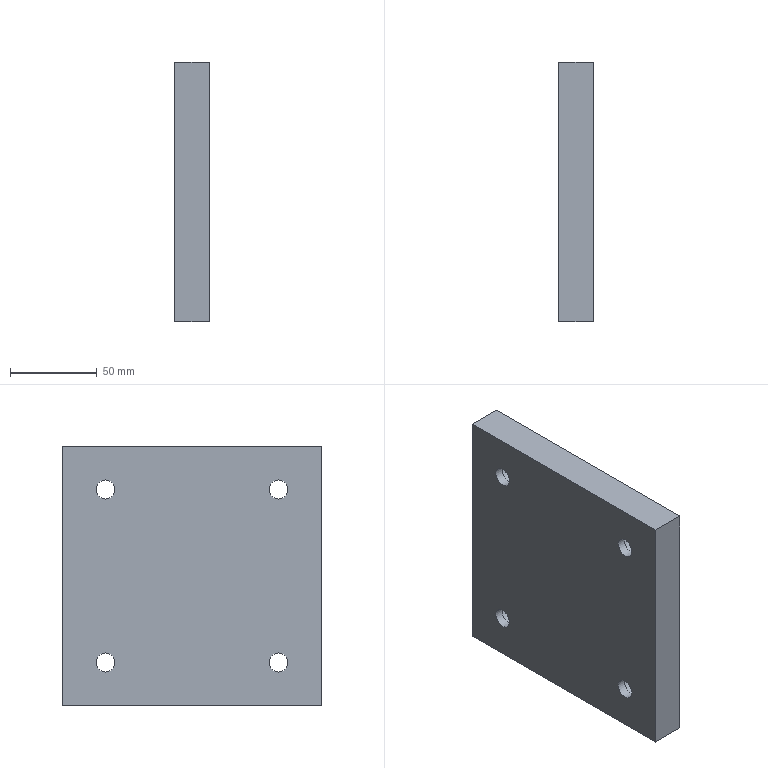Part | NX | features solid 2 | 1 solid | 18 faces | box 20 x 150 x 150 mm | volume 433668 mm3 | plane 10 | cylinder 8 | commonest cylinder face diameters 11 x4 17.5 x4
STEP:
#1=CARTESIAN_POINT('',(1250.,-350.,-256.25));
#2=VERTEX_POINT('',#1);
#3=CARTESIAN_POINT('',(1250.,-350.,-265.));
#4=DIRECTION('',(1.,0.,0.));
#5=DIRECTION('',(0.,0.,1.));
#6=AXIS2_PLACEMENT_3D('',#3,#4,#5);
#7=CIRCLE('',#6,8.75);
#8=EDGE_CURVE('',#2,#2,#7,.T.);
#9=ORIENTED_EDGE('',*,*,#8,.T.);
#10=EDGE_LOOP('',(#9));
#11=FACE_BOUND('',#10,.T.);
#12=CARTESIAN_POINT('',(1250.,-350.,-270.5));
#13=VERTEX_POINT('',#12);
#14=CARTESIAN_POINT('',(1250.,-350.,-265.));
#15=DIRECTION('',(-1.,0.,0.));
#16=DIRECTION('',(0.,0.,-1.));
#17=AXIS2_PLACEMENT_3D('',#14,#15,#16);
#18=CIRCLE('',#17,5.5);
#19=EDGE_CURVE('',#13,#13,#18,.F.);
#20=ORIENTED_EDGE('',*,*,#19,.F.);
#21=EDGE_LOOP('',(#20));
#22=FACE_BOUND('',#21,.T.);
#23=CARTESIAN_POINT('',(1250.,-350.,-265.));
#24=DIRECTION('',(-1.,0.,0.));
#25=DIRECTION('',(0.,0.,-1.));
#26=AXIS2_PLACEMENT_3D('',#23,#24,#25);
#27=PLANE('',#26);
#28=ADVANCED_FACE('',(#11,#22),#27,.F.);
#29=CARTESIAN_POINT('',(1250.,-250.,-256.25));
#30=VERTEX_POINT('',#29);
#31=CARTESIAN_POINT('',(1250.,-250.,-265.));
#32=DIRECTION('',(1.,0.,0.));
#33=DIRECTION('',(0.,0.,1.));
#34=AXIS2_PLACEMENT_3D('',#31,#32,#33);
#35=CIRCLE('',#34,8.75);
#36=EDGE_CURVE('',#30,#30,#35,.T.);
#37=ORIENTED_EDGE('',*,*,#36,.T.);
#38=EDGE_LOOP('',(#37));
#39=FACE_BOUND('',#38,.T.);
#40=CARTESIAN_POINT('',(1250.,-250.,-270.5));
#41=VERTEX_POINT('',#40);
#42=CARTESIAN_POINT('',(1250.,-250.,-265.));
#43=DIRECTION('',(-1.,0.,0.));
#44=DIRECTION('',(0.,0.,-1.));
#45=AXIS2_PLACEMENT_3D('',#42,#43,#44);
#46=CIRCLE('',#45,5.5);
#47=EDGE_CURVE('',#41,#41,#46,.F.);
#48=ORIENTED_EDGE('',*,*,#47,.F.);
#49=EDGE_LOOP('',(#48));
#50=FACE_BOUND('',#49,.T.);
#51=CARTESIAN_POINT('',(1250.,-250.,-265.));
#52=DIRECTION('',(-1.,0.,0.));
#53=DIRECTION('',(0.,0.,-1.));
#54=AXIS2_PLACEMENT_3D('',#51,#52,#53);
#55=PLANE('',#54);
#56=ADVANCED_FACE('',(#39,#50),#55,.F.);
#57=CARTESIAN_POINT('',(1265.,-350.,-273.75));
#58=VERTEX_POINT('',#57);
#59=CARTESIAN_POINT('',(1265.,-350.,-265.));
#60=DIRECTION('',(-1.,0.,0.));
#61=DIRECTION('',(0.,0.,-1.));
#62=AXIS2_PLACEMENT_3D('',#59,#60,#61);
#63=CIRCLE('',#62,8.75);
#64=EDGE_CURVE('',#58,#58,#63,.T.);
#65=ORIENTED_EDGE('',*,*,#64,.F.);
#66=EDGE_LOOP('',(#65));
#67=FACE_BOUND('',#66,.T.);
#68=ORIENTED_EDGE('',*,*,#8,.F.);
#69=EDGE_LOOP('',(#68));
#70=FACE_BOUND('',#69,.T.);
#71=CARTESIAN_POINT('',(1250.,-350.,-265.));
#72=DIRECTION('',(1.,0.,0.));
#73=DIRECTION('',(0.,0.,1.));
#74=AXIS2_PLACEMENT_3D('',#71,#72,#73);
#75=CYLINDRICAL_SURFACE('',#74,8.75);
#76=ADVANCED_FACE('',(#67,#70),#75,.F.);
#77=CARTESIAN_POINT('',(1265.,-250.,-273.75));
#78=VERTEX_POINT('',#77);
#79=CARTESIAN_POINT('',(1265.,-250.,-265.));
#80=DIRECTION('',(-1.,0.,0.));
#81=DIRECTION('',(0.,0.,-1.));
#82=AXIS2_PLACEMENT_3D('',#79,#80,#81);
#83=CIRCLE('',#82,8.75);
#84=EDGE_CURVE('',#78,#78,#83,.T.);
#85=ORIENTED_EDGE('',*,*,#84,.F.);
#86=EDGE_LOOP('',(#85));
#87=FACE_BOUND('',#86,.T.);
#88=ORIENTED_EDGE('',*,*,#36,.F.);
#89=EDGE_LOOP('',(#88));
#90=FACE_BOUND('',#89,.T.);
#91=CARTESIAN_POINT('',(1250.,-250.,-265.));
#92=DIRECTION('',(1.,0.,0.));
#93=DIRECTION('',(0.,0.,1.));
#94=AXIS2_PLACEMENT_3D('',#91,#92,#93);
#95=CYLINDRICAL_SURFACE('',#94,8.75);
#96=ADVANCED_FACE('',(#87,#90),#95,.F.);
#97=CARTESIAN_POINT('',(1245.,-225.,-290.));
#98=VERTEX_POINT('',#97);
#99=CARTESIAN_POINT('',(1245.,-375.,-290.));
#100=VERTEX_POINT('',#99);
#101=CARTESIAN_POINT('',(1245.,-300.,-290.));
#102=DIRECTION('',(0.,-1.,0.));
#103=VECTOR('',#102,1000.);
#104=LINE('',#101,#103);
#105=EDGE_CURVE('',#98,#100,#104,.T.);
#106=ORIENTED_EDGE('',*,*,#105,.F.);
#107=CARTESIAN_POINT('',(1265.,-225.,-290.));
#108=VERTEX_POINT('',#107);
#109=CARTESIAN_POINT('',(1255.,-225.,-290.));
#110=DIRECTION('',(-1.,0.,0.));
#111=VECTOR('',#110,1000.);
#112=LINE('',#109,#111);
#113=EDGE_CURVE('',#108,#98,#112,.T.);
#114=ORIENTED_EDGE('',*,*,#113,.F.);
#115=CARTESIAN_POINT('',(1265.,-375.,-290.));
#116=VERTEX_POINT('',#115);
#117=CARTESIAN_POINT('',(1265.,-300.,-290.));
#118=DIRECTION('',(0.,1.,0.));
#119=VECTOR('',#118,1000.);
#120=LINE('',#117,#119);
#121=EDGE_CURVE('',#116,#108,#120,.T.);
#122=ORIENTED_EDGE('',*,*,#121,.F.);
#123=CARTESIAN_POINT('',(1255.,-375.,-290.));
#124=DIRECTION('',(1.,0.,0.));
#125=VECTOR('',#124,1000.);
#126=LINE('',#123,#125);
#127=EDGE_CURVE('',#100,#116,#126,.T.);
#128=ORIENTED_EDGE('',*,*,#127,.F.);
#129=EDGE_LOOP('',(#106,#114,#122,#128));
#130=FACE_BOUND('',#129,.T.);
#131=CARTESIAN_POINT('',(1255.,-300.,-290.));
#132=DIRECTION('',(0.,0.,-1.));
#133=DIRECTION('',(1.,0.,0.));
#134=AXIS2_PLACEMENT_3D('',#131,#132,#133);
#135=PLANE('',#134);
#136=ADVANCED_FACE('',(#130),#135,.T.);
#137=ORIENTED_EDGE('',*,*,#19,.T.);
#138=EDGE_LOOP('',(#137));
#139=FACE_BOUND('',#138,.T.);
#140=CARTESIAN_POINT('',(1245.,-350.,-259.5));
#141=VERTEX_POINT('',#140);
#142=CARTESIAN_POINT('',(1245.,-350.,-265.));
#143=DIRECTION('',(1.,0.,0.));
#144=DIRECTION('',(0.,0.,1.));
#145=AXIS2_PLACEMENT_3D('',#142,#143,#144);
#146=CIRCLE('',#145,5.5);
#147=EDGE_CURVE('',#141,#141,#146,.T.);
#148=ORIENTED_EDGE('',*,*,#147,.F.);
#149=EDGE_LOOP('',(#148));
#150=FACE_BOUND('',#149,.T.);
#151=CARTESIAN_POINT('',(1245.,-350.,-265.));
#152=DIRECTION('',(1.,0.,0.));
#153=DIRECTION('',(0.,0.,1.));
#154=AXIS2_PLACEMENT_3D('',#151,#152,#153);
#155=CYLINDRICAL_SURFACE('',#154,5.5);
#156=ADVANCED_FACE('',(#139,#150),#155,.F.);
#157=ORIENTED_EDGE('',*,*,#47,.T.);
#158=EDGE_LOOP('',(#157));
#159=FACE_BOUND('',#158,.T.);
#160=CARTESIAN_POINT('',(1245.,-250.,-259.5));
#161=VERTEX_POINT('',#160);
#162=CARTESIAN_POINT('',(1245.,-250.,-265.));
#163=DIRECTION('',(1.,0.,0.));
#164=DIRECTION('',(0.,0.,1.));
#165=AXIS2_PLACEMENT_3D('',#162,#163,#164);
#166=CIRCLE('',#165,5.5);
#167=EDGE_CURVE('',#161,#161,#166,.T.);
#168=ORIENTED_EDGE('',*,*,#167,.F.);
#169=EDGE_LOOP('',(#168));
#170=FACE_BOUND('',#169,.T.);
#171=CARTESIAN_POINT('',(1245.,-250.,-265.));
#172=DIRECTION('',(1.,0.,0.));
#173=DIRECTION('',(0.,0.,1.));
#174=AXIS2_PLACEMENT_3D('',#171,#172,#173);
#175=CYLINDRICAL_SURFACE('',#174,5.5);
#176=ADVANCED_FACE('',(#159,#170),#175,.F.);
#177=ORIENTED_EDGE('',*,*,#167,.T.);
#178=EDGE_LOOP('',(#177));
#179=FACE_BOUND('',#178,.T.);
#180=ORIENTED_EDGE('',*,*,#147,.T.);
#181=EDGE_LOOP('',(#180));
#182=FACE_BOUND('',#181,.T.);
#183=CARTESIAN_POINT('',(1245.,-375.,-140.));
#184=VERTEX_POINT('',#183);
#185=CARTESIAN_POINT('',(1245.,-375.,-290.));
#186=DIRECTION('',(0.,0.,1.));
#187=VECTOR('',#186,1000.);
#188=LINE('',#185,#187);
#189=EDGE_CURVE('',#100,#184,#188,.T.);
#190=ORIENTED_EDGE('',*,*,#189,.T.);
#191=CARTESIAN_POINT('',(1245.,-225.,-140.));
#192=VERTEX_POINT('',#191);
#193=CARTESIAN_POINT('',(1245.,-300.,-140.));
#194=DIRECTION('',(0.,1.,0.));
#195=VECTOR('',#194,1000.);
#196=LINE('',#193,#195);
#197=EDGE_CURVE('',#184,#192,#196,.T.);
#198=ORIENTED_EDGE('',*,*,#197,.T.);
#199=CARTESIAN_POINT('',(1245.,-225.,-290.));
#200=DIRECTION('',(0.,0.,1.));
#201=VECTOR('',#200,1000.);
#202=LINE('',#199,#201);
#203=EDGE_CURVE('',#98,#192,#202,.T.);
#204=ORIENTED_EDGE('',*,*,#203,.F.);
#205=ORIENTED_EDGE('',*,*,#105,.T.);
#206=EDGE_LOOP('',(#190,#198,#204,#205));
#207=FACE_BOUND('',#206,.T.);
#208=CARTESIAN_POINT('',(1245.,-350.,-159.5));
#209=VERTEX_POINT('',#208);
#210=CARTESIAN_POINT('',(1245.,-350.,-165.));
#211=DIRECTION('',(1.,0.,0.));
#212=DIRECTION('',(0.,0.,1.));
#213=AXIS2_PLACEMENT_3D('',#210,#211,#212);
#214=CIRCLE('',#213,5.5);
#215=EDGE_CURVE('',#209,#209,#214,.T.);
#216=ORIENTED_EDGE('',*,*,#215,.T.);
#217=EDGE_LOOP('',(#216));
#218=FACE_BOUND('',#217,.T.);
#219=CARTESIAN_POINT('',(1245.,-250.,-159.5));
#220=VERTEX_POINT('',#219);
#221=CARTESIAN_POINT('',(1245.,-250.,-165.));
#222=DIRECTION('',(1.,0.,0.));
#223=DIRECTION('',(0.,0.,1.));
#224=AXIS2_PLACEMENT_3D('',#221,#222,#223);
#225=CIRCLE('',#224,5.5);
#226=EDGE_CURVE('',#220,#220,#225,.T.);
#227=ORIENTED_EDGE('',*,*,#226,.T.);
#228=EDGE_LOOP('',(#227));
#229=FACE_BOUND('',#228,.T.);
#230=CARTESIAN_POINT('',(1245.,-300.,-290.));
#231=DIRECTION('',(-1.,0.,0.));
#232=DIRECTION('',(0.,0.,-1.));
#233=AXIS2_PLACEMENT_3D('',#230,#231,#232);
#234=PLANE('',#233);
#235=ADVANCED_FACE('',(#179,#182,#207,#218,#229),#234,.T.);
#236=CARTESIAN_POINT('',(1265.,-375.,-140.));
#237=VERTEX_POINT('',#236);
#238=CARTESIAN_POINT('',(1265.,-375.,-290.));
#239=DIRECTION('',(0.,0.,1.));
#240=VECTOR('',#239,1000.);
#241=LINE('',#238,#240);
#242=EDGE_CURVE('',#116,#237,#241,.T.);
#243=ORIENTED_EDGE('',*,*,#242,.T.);
#244=CARTESIAN_POINT('',(1255.,-375.,-140.));
#245=DIRECTION('',(-1.,0.,0.));
#246=VECTOR('',#245,1000.);
#247=LINE('',#244,#246);
#248=EDGE_CURVE('',#237,#184,#247,.T.);
#249=ORIENTED_EDGE('',*,*,#248,.T.);
#250=ORIENTED_EDGE('',*,*,#189,.F.);
#251=ORIENTED_EDGE('',*,*,#127,.T.);
#252=EDGE_LOOP('',(#243,#249,#250,#251));
#253=FACE_BOUND('',#252,.T.);
#254=CARTESIAN_POINT('',(1255.,-375.,-290.));
#255=DIRECTION('',(0.,-1.,0.));
#256=DIRECTION('',(0.,0.,1.));
#257=AXIS2_PLACEMENT_3D('',#254,#255,#256);
#258=PLANE('',#257);
#259=ADVANCED_FACE('',(#253),#258,.T.);
#260=ORIENTED_EDGE('',*,*,#84,.T.);
#261=EDGE_LOOP('',(#260));
#262=FACE_BOUND('',#261,.T.);
#263=ORIENTED_EDGE('',*,*,#64,.T.);
#264=EDGE_LOOP('',(#263));
#265=FACE_BOUND('',#264,.T.);
#266=CARTESIAN_POINT('',(1265.,-225.,-140.));
#267=VERTEX_POINT('',#266);
#268=CARTESIAN_POINT('',(1265.,-225.,-290.));
#269=DIRECTION('',(0.,0.,1.));
#270=VECTOR('',#269,1000.);
#271=LINE('',#268,#270);
#272=EDGE_CURVE('',#108,#267,#271,.T.);
#273=ORIENTED_EDGE('',*,*,#272,.T.);
#274=CARTESIAN_POINT('',(1265.,-300.,-140.));
#275=DIRECTION('',(0.,-1.,0.));
#276=VECTOR('',#275,1000.);
#277=LINE('',#274,#276);
#278=EDGE_CURVE('',#267,#237,#277,.T.);
#279=ORIENTED_EDGE('',*,*,#278,.T.);
#280=ORIENTED_EDGE('',*,*,#242,.F.);
#281=ORIENTED_EDGE('',*,*,#121,.T.);
#282=EDGE_LOOP('',(#273,#279,#280,#281));
#283=FACE_BOUND('',#282,.T.);
#284=CARTESIAN_POINT('',(1265.,-350.,-173.75));
#285=VERTEX_POINT('',#284);
#286=CARTESIAN_POINT('',(1265.,-350.,-165.));
#287=DIRECTION('',(-1.,0.,0.));
#288=DIRECTION('',(0.,0.,-1.));
#289=AXIS2_PLACEMENT_3D('',#286,#287,#288);
#290=CIRCLE('',#289,8.75);
#291=EDGE_CURVE('',#285,#285,#290,.T.);
#292=ORIENTED_EDGE('',*,*,#291,.T.);
#293=EDGE_LOOP('',(#292));
#294=FACE_BOUND('',#293,.T.);
#295=CARTESIAN_POINT('',(1265.,-250.,-173.75));
#296=VERTEX_POINT('',#295);
#297=CARTESIAN_POINT('',(1265.,-250.,-165.));
#298=DIRECTION('',(-1.,0.,0.));
#299=DIRECTION('',(0.,0.,-1.));
#300=AXIS2_PLACEMENT_3D('',#297,#298,#299);
#301=CIRCLE('',#300,8.75);
#302=EDGE_CURVE('',#296,#296,#301,.T.);
#303=ORIENTED_EDGE('',*,*,#302,.T.);
#304=EDGE_LOOP('',(#303));
#305=FACE_BOUND('',#304,.T.);
#306=CARTESIAN_POINT('',(1265.,-300.,-290.));
#307=DIRECTION('',(1.,0.,0.));
#308=DIRECTION('',(0.,0.,1.));
#309=AXIS2_PLACEMENT_3D('',#306,#307,#308);
#310=PLANE('',#309);
#311=ADVANCED_FACE('',(#262,#265,#283,#294,#305),#310,.T.);
#312=ORIENTED_EDGE('',*,*,#203,.T.);
#313=CARTESIAN_POINT('',(1255.,-225.,-140.));
#314=DIRECTION('',(1.,0.,0.));
#315=VECTOR('',#314,1000.);
#316=LINE('',#313,#315);
#317=EDGE_CURVE('',#192,#267,#316,.T.);
#318=ORIENTED_EDGE('',*,*,#317,.T.);
#319=ORIENTED_EDGE('',*,*,#272,.F.);
#320=ORIENTED_EDGE('',*,*,#113,.T.);
#321=EDGE_LOOP('',(#312,#318,#319,#320));
#322=FACE_BOUND('',#321,.T.);
#323=CARTESIAN_POINT('',(1255.,-225.,-290.));
#324=DIRECTION('',(0.,1.,0.));
#325=DIRECTION('',(0.,0.,-1.));
#326=AXIS2_PLACEMENT_3D('',#323,#324,#325);
#327=PLANE('',#326);
#328=ADVANCED_FACE('',(#322),#327,.T.);
#329=ORIENTED_EDGE('',*,*,#317,.F.);
#330=ORIENTED_EDGE('',*,*,#197,.F.);
#331=ORIENTED_EDGE('',*,*,#248,.F.);
#332=ORIENTED_EDGE('',*,*,#278,.F.);
#333=EDGE_LOOP('',(#329,#330,#331,#332));
#334=FACE_BOUND('',#333,.T.);
#335=CARTESIAN_POINT('',(1255.,-300.,-140.));
#336=DIRECTION('',(0.,0.,1.));
#337=DIRECTION('',(-1.,0.,0.));
#338=AXIS2_PLACEMENT_3D('',#335,#336,#337);
#339=PLANE('',#338);
#340=ADVANCED_FACE('',(#334),#339,.T.);
#341=CARTESIAN_POINT('',(1250.,-250.,-170.5));
#342=VERTEX_POINT('',#341);
#343=CARTESIAN_POINT('',(1250.,-250.,-165.));
#344=DIRECTION('',(-1.,0.,0.));
#345=DIRECTION('',(0.,0.,-1.));
#346=AXIS2_PLACEMENT_3D('',#343,#344,#345);
#347=CIRCLE('',#346,5.5);
#348=EDGE_CURVE('',#342,#342,#347,.F.);
#349=ORIENTED_EDGE('',*,*,#348,.T.);
#350=EDGE_LOOP('',(#349));
#351=FACE_BOUND('',#350,.T.);
#352=ORIENTED_EDGE('',*,*,#226,.F.);
#353=EDGE_LOOP('',(#352));
#354=FACE_BOUND('',#353,.T.);
#355=CARTESIAN_POINT('',(1245.,-250.,-165.));
#356=DIRECTION('',(1.,0.,0.));
#357=DIRECTION('',(0.,0.,1.));
#358=AXIS2_PLACEMENT_3D('',#355,#356,#357);
#359=CYLINDRICAL_SURFACE('',#358,5.5);
#360=ADVANCED_FACE('',(#351,#354),#359,.F.);
#361=CARTESIAN_POINT('',(1250.,-250.,-156.25));
#362=VERTEX_POINT('',#361);
#363=CARTESIAN_POINT('',(1250.,-250.,-165.));
#364=DIRECTION('',(1.,0.,0.));
#365=DIRECTION('',(0.,0.,1.));
#366=AXIS2_PLACEMENT_3D('',#363,#364,#365);
#367=CIRCLE('',#366,8.75);
#368=EDGE_CURVE('',#362,#362,#367,.T.);
#369=ORIENTED_EDGE('',*,*,#368,.T.);
#370=EDGE_LOOP('',(#369));
#371=FACE_BOUND('',#370,.T.);
#372=ORIENTED_EDGE('',*,*,#348,.F.);
#373=EDGE_LOOP('',(#372));
#374=FACE_BOUND('',#373,.T.);
#375=CARTESIAN_POINT('',(1250.,-250.,-165.));
#376=DIRECTION('',(-1.,0.,0.));
#377=DIRECTION('',(0.,0.,-1.));
#378=AXIS2_PLACEMENT_3D('',#375,#376,#377);
#379=PLANE('',#378);
#380=ADVANCED_FACE('',(#371,#374),#379,.F.);
#381=ORIENTED_EDGE('',*,*,#302,.F.);
#382=EDGE_LOOP('',(#381));
#383=FACE_BOUND('',#382,.T.);
#384=ORIENTED_EDGE('',*,*,#368,.F.);
#385=EDGE_LOOP('',(#384));
#386=FACE_BOUND('',#385,.T.);
#387=CARTESIAN_POINT('',(1250.,-250.,-165.));
#388=DIRECTION('',(1.,0.,0.));
#389=DIRECTION('',(0.,0.,1.));
#390=AXIS2_PLACEMENT_3D('',#387,#388,#389);
#391=CYLINDRICAL_SURFACE('',#390,8.75);
#392=ADVANCED_FACE('',(#383,#386),#391,.F.);
#393=CARTESIAN_POINT('',(1250.,-350.,-170.5));
#394=VERTEX_POINT('',#393);
#395=CARTESIAN_POINT('',(1250.,-350.,-165.));
#396=DIRECTION('',(-1.,0.,0.));
#397=DIRECTION('',(0.,0.,-1.));
#398=AXIS2_PLACEMENT_3D('',#395,#396,#397);
#399=CIRCLE('',#398,5.5);
#400=EDGE_CURVE('',#394,#394,#399,.F.);
#401=ORIENTED_EDGE('',*,*,#400,.T.);
#402=EDGE_LOOP('',(#401));
#403=FACE_BOUND('',#402,.T.);
#404=ORIENTED_EDGE('',*,*,#215,.F.);
#405=EDGE_LOOP('',(#404));
#406=FACE_BOUND('',#405,.T.);
#407=CARTESIAN_POINT('',(1245.,-350.,-165.));
#408=DIRECTION('',(1.,0.,0.));
#409=DIRECTION('',(0.,0.,1.));
#410=AXIS2_PLACEMENT_3D('',#407,#408,#409);
#411=CYLINDRICAL_SURFACE('',#410,5.5);
#412=ADVANCED_FACE('',(#403,#406),#411,.F.);
#413=CARTESIAN_POINT('',(1250.,-350.,-156.25));
#414=VERTEX_POINT('',#413);
#415=CARTESIAN_POINT('',(1250.,-350.,-165.));
#416=DIRECTION('',(1.,0.,0.));
#417=DIRECTION('',(0.,0.,1.));
#418=AXIS2_PLACEMENT_3D('',#415,#416,#417);
#419=CIRCLE('',#418,8.75);
#420=EDGE_CURVE('',#414,#414,#419,.T.);
#421=ORIENTED_EDGE('',*,*,#420,.T.);
#422=EDGE_LOOP('',(#421));
#423=FACE_BOUND('',#422,.T.);
#424=ORIENTED_EDGE('',*,*,#400,.F.);
#425=EDGE_LOOP('',(#424));
#426=FACE_BOUND('',#425,.T.);
#427=CARTESIAN_POINT('',(1250.,-350.,-165.));
#428=DIRECTION('',(-1.,0.,0.));
#429=DIRECTION('',(0.,0.,-1.));
#430=AXIS2_PLACEMENT_3D('',#427,#428,#429);
#431=PLANE('',#430);
#432=ADVANCED_FACE('',(#423,#426),#431,.F.);
#433=ORIENTED_EDGE('',*,*,#291,.F.);
#434=EDGE_LOOP('',(#433));
#435=FACE_BOUND('',#434,.T.);
#436=ORIENTED_EDGE('',*,*,#420,.F.);
#437=EDGE_LOOP('',(#436));
#438=FACE_BOUND('',#437,.T.);
#439=CARTESIAN_POINT('',(1250.,-350.,-165.));
#440=DIRECTION('',(1.,0.,0.));
#441=DIRECTION('',(0.,0.,1.));
#442=AXIS2_PLACEMENT_3D('',#439,#440,#441);
#443=CYLINDRICAL_SURFACE('',#442,8.75);
#444=ADVANCED_FACE('',(#435,#438),#443,.F.);
#445=CLOSED_SHELL('',(#28,#56,#76,#96,#136,#156,#176,#235,#259,#311,#328,#340,#360,#380,#392,#412,#432,#444));
#446=MANIFOLD_SOLID_BREP('',#445);
#447=(LENGTH_UNIT()NAMED_UNIT(*)SI_UNIT(.MILLI.,.METRE.));
#448=UNCERTAINTY_MEASURE_WITH_UNIT(LENGTH_MEASURE(0.00001),#447,'','');
#449=(NAMED_UNIT(*)PLANE_ANGLE_UNIT()SI_UNIT($,.RADIAN.));
#450=(NAMED_UNIT(*)SI_UNIT($,.STERADIAN.)SOLID_ANGLE_UNIT());
#451=(GEOMETRIC_REPRESENTATION_CONTEXT(3)GLOBAL_UNCERTAINTY_ASSIGNED_CONTEXT((#448))GLOBAL_UNIT_ASSIGNED_CONTEXT((#447,#449,#450))REPRESENTATION_CONTEXT('',''));
#452=ADVANCED_BREP_SHAPE_REPRESENTATION('',(#446),#451);